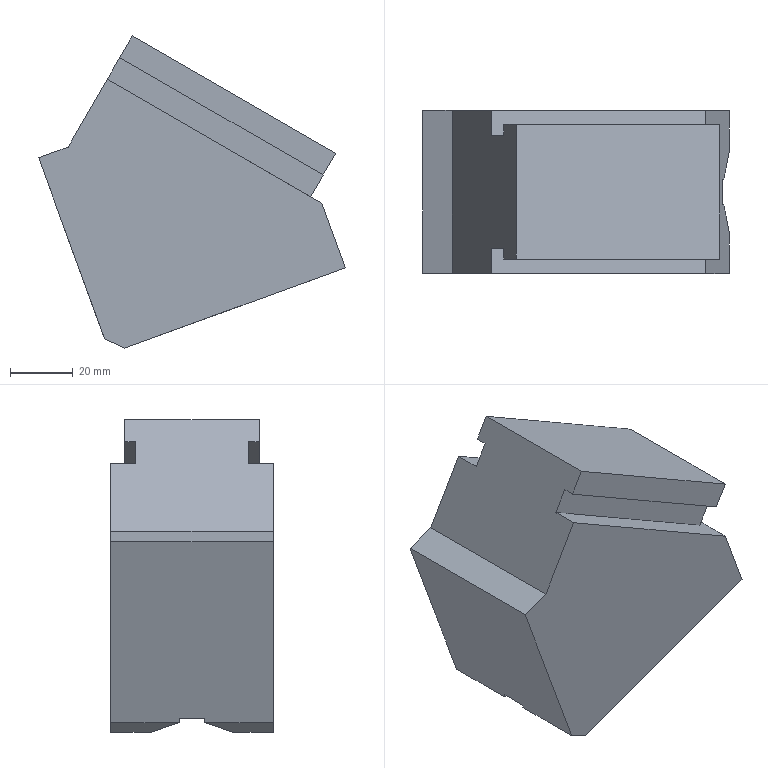Part | NX | features solid 2 | 1 solid | 32 faces | box 97.92 x 52 x 99.707 mm | volume 275545 mm3 | plane 30 | cylinder 2 | commonest cylinder face diameters 20 x2
STEP:
#1=CARTESIAN_POINT('',(-458.531,-112.,17.471));
#2=VERTEX_POINT('',#1);
#3=CARTESIAN_POINT('',(-458.531,-148.,17.471));
#4=VERTEX_POINT('',#3);
#5=CARTESIAN_POINT('',(-458.531,-112.,17.471));
#6=DIRECTION('',(0.,-1.,0.));
#7=VECTOR('',#6,1000.);
#8=LINE('',#5,#7);
#9=EDGE_CURVE('',#2,#4,#8,.T.);
#10=ORIENTED_EDGE('',*,*,#9,.T.);
#11=CARTESIAN_POINT('',(-523.483,-148.,54.971));
#12=VERTEX_POINT('',#11);
#13=CARTESIAN_POINT('',(-458.531,-148.,17.471));
#14=DIRECTION('',(-0.866,0.,0.5));
#15=VECTOR('',#14,1000.);
#16=LINE('',#13,#15);
#17=EDGE_CURVE('',#4,#12,#16,.T.);
#18=ORIENTED_EDGE('',*,*,#17,.T.);
#19=CARTESIAN_POINT('',(-523.483,-156.,54.971));
#20=VERTEX_POINT('',#19);
#21=CARTESIAN_POINT('',(-523.483,-156.,54.971));
#22=DIRECTION('',(0.,1.,0.));
#23=VECTOR('',#22,1000.);
#24=LINE('',#21,#23);
#25=EDGE_CURVE('',#20,#12,#24,.T.);
#26=ORIENTED_EDGE('',*,*,#25,.F.);
#27=CARTESIAN_POINT('',(-454.975,-156.,15.417));
#28=VERTEX_POINT('',#27);
#29=CARTESIAN_POINT('',(-454.975,-156.,15.417));
#30=DIRECTION('',(-0.866,0.,0.5));
#31=VECTOR('',#30,1000.);
#32=LINE('',#29,#31);
#33=EDGE_CURVE('',#28,#20,#32,.T.);
#34=ORIENTED_EDGE('',*,*,#33,.F.);
#35=CARTESIAN_POINT('',(-454.975,-104.,15.417));
#36=VERTEX_POINT('',#35);
#37=CARTESIAN_POINT('',(-454.975,-156.,15.417));
#38=DIRECTION('',(0.,1.,0.));
#39=VECTOR('',#38,1000.);
#40=LINE('',#37,#39);
#41=EDGE_CURVE('',#28,#36,#40,.T.);
#42=ORIENTED_EDGE('',*,*,#41,.T.);
#43=CARTESIAN_POINT('',(-523.483,-104.,54.971));
#44=VERTEX_POINT('',#43);
#45=CARTESIAN_POINT('',(-454.975,-104.,15.417));
#46=DIRECTION('',(-0.866,0.,0.5));
#47=VECTOR('',#46,1000.);
#48=LINE('',#45,#47);
#49=EDGE_CURVE('',#36,#44,#48,.T.);
#50=ORIENTED_EDGE('',*,*,#49,.T.);
#51=CARTESIAN_POINT('',(-523.483,-112.,54.971));
#52=VERTEX_POINT('',#51);
#53=CARTESIAN_POINT('',(-523.483,-156.,54.971));
#54=DIRECTION('',(0.,1.,0.));
#55=VECTOR('',#54,1000.);
#56=LINE('',#53,#55);
#57=EDGE_CURVE('',#52,#44,#56,.T.);
#58=ORIENTED_EDGE('',*,*,#57,.F.);
#59=CARTESIAN_POINT('',(-458.531,-112.,17.471));
#60=DIRECTION('',(-0.866,0.,0.5));
#61=VECTOR('',#60,1000.);
#62=LINE('',#59,#61);
#63=EDGE_CURVE('',#2,#52,#62,.T.);
#64=ORIENTED_EDGE('',*,*,#63,.F.);
#65=EDGE_LOOP('',(#10,#18,#26,#34,#42,#50,#58,#64));
#66=FACE_BOUND('',#65,.T.);
#67=CARTESIAN_POINT('',(-454.975,-156.,15.417));
#68=DIRECTION('',(0.5,0.,0.866));
#69=DIRECTION('',(-0.866,0.,0.5));
#70=AXIS2_PLACEMENT_3D('',#67,#68,#69);
#71=PLANE('',#70);
#72=ADVANCED_FACE('',(#66),#71,.T.);
#73=CARTESIAN_POINT('',(-517.937,-142.99,-30.879));
#74=VERTEX_POINT('',#73);
#75=CARTESIAN_POINT('',(-447.46,-142.99,-5.228));
#76=VERTEX_POINT('',#75);
#77=CARTESIAN_POINT('',(-447.46,-142.99,-5.228));
#78=DIRECTION('',(0.9397,0.,0.342));
#79=VECTOR('',#78,1000.);
#80=LINE('',#77,#79);
#81=EDGE_CURVE('',#74,#76,#80,.T.);
#82=ORIENTED_EDGE('',*,*,#81,.T.);
#83=CARTESIAN_POINT('',(-447.46,-156.,-5.228));
#84=VERTEX_POINT('',#83);
#85=CARTESIAN_POINT('',(-447.46,-156.,-5.228));
#86=DIRECTION('',(0.,1.,0.));
#87=VECTOR('',#86,1000.);
#88=LINE('',#85,#87);
#89=EDGE_CURVE('',#84,#76,#88,.T.);
#90=ORIENTED_EDGE('',*,*,#89,.F.);
#91=CARTESIAN_POINT('',(-517.937,-156.,-30.879));
#92=VERTEX_POINT('',#91);
#93=CARTESIAN_POINT('',(-447.46,-156.,-5.228));
#94=DIRECTION('',(-0.9397,0.,-0.342));
#95=VECTOR('',#94,1000.);
#96=LINE('',#93,#95);
#97=EDGE_CURVE('',#84,#92,#96,.T.);
#98=ORIENTED_EDGE('',*,*,#97,.T.);
#99=CARTESIAN_POINT('',(-517.937,-156.,-30.879));
#100=DIRECTION('',(0.,-1.,0.));
#101=VECTOR('',#100,1000.);
#102=LINE('',#99,#101);
#103=EDGE_CURVE('',#74,#92,#102,.T.);
#104=ORIENTED_EDGE('',*,*,#103,.F.);
#105=EDGE_LOOP('',(#82,#90,#98,#104));
#106=FACE_BOUND('',#105,.T.);
#107=CARTESIAN_POINT('',(-447.46,-156.,-5.228));
#108=DIRECTION('',(-0.342,0.,0.9397));
#109=DIRECTION('',(-0.9397,0.,-0.342));
#110=AXIS2_PLACEMENT_3D('',#107,#108,#109);
#111=PLANE('',#110);
#112=ADVANCED_FACE('',(#106),#111,.F.);
#113=CARTESIAN_POINT('',(-449.236,-134.,-0.3504));
#114=VERTEX_POINT('',#113);
#115=CARTESIAN_POINT('',(-449.236,-134.,-0.3504));
#116=DIRECTION('',(0.171,-0.866,-0.4698));
#117=VECTOR('',#116,1000.);
#118=LINE('',#115,#117);
#119=EDGE_CURVE('',#114,#76,#118,.T.);
#120=ORIENTED_EDGE('',*,*,#119,.F.);
#121=CARTESIAN_POINT('',(-449.683,-134.,0.8801));
#122=VERTEX_POINT('',#121);
#123=CARTESIAN_POINT('',(-449.683,-134.,0.8801));
#124=DIRECTION('',(0.342,0.,-0.9397));
#125=VECTOR('',#124,1000.);
#126=LINE('',#123,#125);
#127=EDGE_CURVE('',#122,#114,#126,.T.);
#128=ORIENTED_EDGE('',*,*,#127,.F.);
#129=CARTESIAN_POINT('',(-449.683,-126.,0.8801));
#130=VERTEX_POINT('',#129);
#131=CARTESIAN_POINT('',(-449.683,-134.,0.8801));
#132=DIRECTION('',(0.,1.,0.));
#133=VECTOR('',#132,1000.);
#134=LINE('',#131,#133);
#135=EDGE_CURVE('',#122,#130,#134,.T.);
#136=ORIENTED_EDGE('',*,*,#135,.T.);
#137=CARTESIAN_POINT('',(-449.236,-126.,-0.3504));
#138=VERTEX_POINT('',#137);
#139=CARTESIAN_POINT('',(-449.236,-126.,-0.3504));
#140=DIRECTION('',(-0.342,0.,0.9397));
#141=VECTOR('',#140,1000.);
#142=LINE('',#139,#141);
#143=EDGE_CURVE('',#138,#130,#142,.T.);
#144=ORIENTED_EDGE('',*,*,#143,.F.);
#145=CARTESIAN_POINT('',(-447.46,-117.01,-5.228));
#146=VERTEX_POINT('',#145);
#147=CARTESIAN_POINT('',(-447.46,-117.01,-5.228));
#148=DIRECTION('',(0.171,0.866,-0.4698));
#149=VECTOR('',#148,1000.);
#150=LINE('',#147,#149);
#151=EDGE_CURVE('',#138,#146,#150,.T.);
#152=ORIENTED_EDGE('',*,*,#151,.T.);
#153=CARTESIAN_POINT('',(-447.46,-104.,-5.228));
#154=VERTEX_POINT('',#153);
#155=CARTESIAN_POINT('',(-447.46,-156.,-5.228));
#156=DIRECTION('',(0.,1.,0.));
#157=VECTOR('',#156,1000.);
#158=LINE('',#155,#157);
#159=EDGE_CURVE('',#146,#154,#158,.T.);
#160=ORIENTED_EDGE('',*,*,#159,.T.);
#161=CARTESIAN_POINT('',(-454.975,-104.,15.417));
#162=DIRECTION('',(0.342,0.,-0.9397));
#163=VECTOR('',#162,1000.);
#164=LINE('',#161,#163);
#165=EDGE_CURVE('',#36,#154,#164,.T.);
#166=ORIENTED_EDGE('',*,*,#165,.F.);
#167=ORIENTED_EDGE('',*,*,#41,.F.);
#168=CARTESIAN_POINT('',(-454.975,-156.,15.417));
#169=DIRECTION('',(0.342,0.,-0.9397));
#170=VECTOR('',#169,1000.);
#171=LINE('',#168,#170);
#172=EDGE_CURVE('',#28,#84,#171,.T.);
#173=ORIENTED_EDGE('',*,*,#172,.T.);
#174=ORIENTED_EDGE('',*,*,#89,.T.);
#175=EDGE_LOOP('',(#120,#128,#136,#144,#152,#160,#166,#167,#173,#174));
#176=FACE_BOUND('',#175,.T.);
#177=CARTESIAN_POINT('',(-454.975,-156.,15.417));
#178=DIRECTION('',(-0.9397,0.,-0.342));
#179=DIRECTION('',(0.342,0.,-0.9397));
#180=AXIS2_PLACEMENT_3D('',#177,#178,#179);
#181=PLANE('',#180);
#182=ADVANCED_FACE('',(#176),#181,.F.);
#183=CARTESIAN_POINT('',(-524.346,-125.67,-27.891));
#184=VERTEX_POINT('',#183);
#185=CARTESIAN_POINT('',(-524.411,-126.,-27.712));
#186=VERTEX_POINT('',#185);
#187=CARTESIAN_POINT('',(-534.096,-175.048,-1.102));
#188=DIRECTION('',(-0.171,-0.866,0.4698));
#189=VECTOR('',#188,1000.);
#190=LINE('',#187,#189);
#191=EDGE_CURVE('',#184,#186,#190,.T.);
#192=ORIENTED_EDGE('',*,*,#191,.T.);
#193=CARTESIAN_POINT('',(-524.859,-126.,-26.482));
#194=VERTEX_POINT('',#193);
#195=CARTESIAN_POINT('',(-545.38,-126.,29.9));
#196=DIRECTION('',(0.342,0.,-0.9397));
#197=VECTOR('',#196,1000.);
#198=LINE('',#195,#197);
#199=EDGE_CURVE('',#194,#186,#198,.T.);
#200=ORIENTED_EDGE('',*,*,#199,.F.);
#201=CARTESIAN_POINT('',(-524.859,-134.,-26.482));
#202=VERTEX_POINT('',#201);
#203=CARTESIAN_POINT('',(-524.859,-156.,-26.482));
#204=DIRECTION('',(0.,-1.,0.));
#205=VECTOR('',#204,1000.);
#206=LINE('',#203,#205);
#207=EDGE_CURVE('',#194,#202,#206,.T.);
#208=ORIENTED_EDGE('',*,*,#207,.T.);
#209=CARTESIAN_POINT('',(-524.411,-134.,-27.712));
#210=VERTEX_POINT('',#209);
#211=CARTESIAN_POINT('',(-545.38,-134.,29.9));
#212=DIRECTION('',(-0.342,0.,0.9397));
#213=VECTOR('',#212,1000.);
#214=LINE('',#211,#213);
#215=EDGE_CURVE('',#210,#202,#214,.T.);
#216=ORIENTED_EDGE('',*,*,#215,.F.);
#217=CARTESIAN_POINT('',(-524.346,-134.33,-27.891));
#218=VERTEX_POINT('',#217);
#219=CARTESIAN_POINT('',(-526.395,-123.952,-22.261));
#220=DIRECTION('',(-0.171,0.866,0.4698));
#221=VECTOR('',#220,1000.);
#222=LINE('',#219,#221);
#223=EDGE_CURVE('',#218,#210,#222,.T.);
#224=ORIENTED_EDGE('',*,*,#223,.F.);
#225=CARTESIAN_POINT('',(-524.346,-156.,-27.891));
#226=VERTEX_POINT('',#225);
#227=CARTESIAN_POINT('',(-524.346,-142.99,-27.891));
#228=DIRECTION('',(0.,1.,0.));
#229=VECTOR('',#228,1000.);
#230=LINE('',#227,#229);
#231=EDGE_CURVE('',#226,#218,#230,.T.);
#232=ORIENTED_EDGE('',*,*,#231,.F.);
#233=CARTESIAN_POINT('',(-545.38,-156.,29.9));
#234=VERTEX_POINT('',#233);
#235=CARTESIAN_POINT('',(-545.38,-156.,29.9));
#236=DIRECTION('',(0.342,0.,-0.9397));
#237=VECTOR('',#236,1000.);
#238=LINE('',#235,#237);
#239=EDGE_CURVE('',#234,#226,#238,.T.);
#240=ORIENTED_EDGE('',*,*,#239,.F.);
#241=CARTESIAN_POINT('',(-545.38,-104.,29.9));
#242=VERTEX_POINT('',#241);
#243=CARTESIAN_POINT('',(-545.38,-156.,29.9));
#244=DIRECTION('',(0.,1.,0.));
#245=VECTOR('',#244,1000.);
#246=LINE('',#243,#245);
#247=EDGE_CURVE('',#234,#242,#246,.T.);
#248=ORIENTED_EDGE('',*,*,#247,.T.);
#249=CARTESIAN_POINT('',(-524.346,-104.,-27.891));
#250=VERTEX_POINT('',#249);
#251=CARTESIAN_POINT('',(-545.38,-104.,29.9));
#252=DIRECTION('',(0.342,0.,-0.9397));
#253=VECTOR('',#252,1000.);
#254=LINE('',#251,#253);
#255=EDGE_CURVE('',#242,#250,#254,.T.);
#256=ORIENTED_EDGE('',*,*,#255,.T.);
#257=CARTESIAN_POINT('',(-524.346,-104.,-27.891));
#258=DIRECTION('',(0.,1.,0.));
#259=VECTOR('',#258,1000.);
#260=LINE('',#257,#259);
#261=EDGE_CURVE('',#184,#250,#260,.T.);
#262=ORIENTED_EDGE('',*,*,#261,.F.);
#263=EDGE_LOOP('',(#192,#200,#208,#216,#224,#232,#240,#248,#256,#262));
#264=FACE_BOUND('',#263,.T.);
#265=CARTESIAN_POINT('',(-545.38,-156.,29.9));
#266=DIRECTION('',(-0.9397,0.,-0.342));
#267=DIRECTION('',(0.342,0.,-0.9397));
#268=AXIS2_PLACEMENT_3D('',#265,#266,#267);
#269=PLANE('',#268);
#270=ADVANCED_FACE('',(#264),#269,.T.);
#271=ORIENTED_EDGE('',*,*,#255,.F.);
#272=CARTESIAN_POINT('',(-535.983,-104.,33.32));
#273=VERTEX_POINT('',#272);
#274=CARTESIAN_POINT('',(-535.983,-104.,33.32));
#275=DIRECTION('',(-0.9397,0.,-0.342));
#276=VECTOR('',#275,1000.);
#277=LINE('',#274,#276);
#278=EDGE_CURVE('',#273,#242,#277,.T.);
#279=ORIENTED_EDGE('',*,*,#278,.F.);
#280=CARTESIAN_POINT('',(-523.483,-104.,54.971));
#281=DIRECTION('',(-0.5,0.,-0.866));
#282=VECTOR('',#281,1000.);
#283=LINE('',#280,#282);
#284=EDGE_CURVE('',#44,#273,#283,.T.);
#285=ORIENTED_EDGE('',*,*,#284,.F.);
#286=ORIENTED_EDGE('',*,*,#49,.F.);
#287=ORIENTED_EDGE('',*,*,#165,.T.);
#288=CARTESIAN_POINT('',(-473.862,-104.,-14.837));
#289=VERTEX_POINT('',#288);
#290=CARTESIAN_POINT('',(-447.46,-104.,-5.228));
#291=DIRECTION('',(-0.9397,0.,-0.342));
#292=VECTOR('',#291,1000.);
#293=LINE('',#290,#292);
#294=EDGE_CURVE('',#154,#289,#293,.T.);
#295=ORIENTED_EDGE('',*,*,#294,.T.);
#296=CARTESIAN_POINT('',(-479.59,-104.,0.8997));
#297=VERTEX_POINT('',#296);
#298=CARTESIAN_POINT('',(-486.43,-104.,19.694));
#299=DIRECTION('',(0.342,0.,-0.9397));
#300=VECTOR('',#299,1000.);
#301=LINE('',#298,#300);
#302=EDGE_CURVE('',#297,#289,#301,.T.);
#303=ORIENTED_EDGE('',*,*,#302,.F.);
#304=CARTESIAN_POINT('',(-486.43,-104.,19.694));
#305=VERTEX_POINT('',#304);
#306=CARTESIAN_POINT('',(-483.01,-104.,10.297));
#307=DIRECTION('',(0.,1.,0.));
#308=DIRECTION('',(-1.,0.,0.));
#309=AXIS2_PLACEMENT_3D('',#306,#307,#308);
#310=CIRCLE('',#309,10.);
#311=EDGE_CURVE('',#305,#297,#310,.T.);
#312=ORIENTED_EDGE('',*,*,#311,.F.);
#313=CARTESIAN_POINT('',(-505.224,-104.,12.853));
#314=VERTEX_POINT('',#313);
#315=CARTESIAN_POINT('',(-505.224,-104.,12.853));
#316=DIRECTION('',(0.9397,0.,0.342));
#317=VECTOR('',#316,1000.);
#318=LINE('',#315,#317);
#319=EDGE_CURVE('',#314,#305,#318,.T.);
#320=ORIENTED_EDGE('',*,*,#319,.F.);
#321=CARTESIAN_POINT('',(-498.383,-104.,-5.941));
#322=VERTEX_POINT('',#321);
#323=CARTESIAN_POINT('',(-501.804,-104.,3.456));
#324=DIRECTION('',(0.,1.,0.));
#325=DIRECTION('',(-1.,0.,0.));
#326=AXIS2_PLACEMENT_3D('',#323,#324,#325);
#327=CIRCLE('',#326,10.);
#328=EDGE_CURVE('',#322,#314,#327,.T.);
#329=ORIENTED_EDGE('',*,*,#328,.F.);
#330=CARTESIAN_POINT('',(-492.656,-104.,-21.678));
#331=VERTEX_POINT('',#330);
#332=CARTESIAN_POINT('',(-505.224,-104.,12.853));
#333=DIRECTION('',(0.342,0.,-0.9397));
#334=VECTOR('',#333,1000.);
#335=LINE('',#332,#334);
#336=EDGE_CURVE('',#322,#331,#335,.T.);
#337=ORIENTED_EDGE('',*,*,#336,.T.);
#338=CARTESIAN_POINT('',(-517.937,-104.,-30.879));
#339=VERTEX_POINT('',#338);
#340=CARTESIAN_POINT('',(-447.46,-104.,-5.228));
#341=DIRECTION('',(-0.9397,0.,-0.342));
#342=VECTOR('',#341,1000.);
#343=LINE('',#340,#342);
#344=EDGE_CURVE('',#331,#339,#343,.T.);
#345=ORIENTED_EDGE('',*,*,#344,.T.);
#346=CARTESIAN_POINT('',(-524.346,-104.,-27.891));
#347=DIRECTION('',(0.9063,0.,-0.4226));
#348=VECTOR('',#347,1000.);
#349=LINE('',#346,#348);
#350=EDGE_CURVE('',#250,#339,#349,.T.);
#351=ORIENTED_EDGE('',*,*,#350,.F.);
#352=EDGE_LOOP('',(#271,#279,#285,#286,#287,#295,#303,#312,#320,#329,#337,#345,#351));
#353=FACE_BOUND('',#352,.T.);
#354=CARTESIAN_POINT('',(-447.46,-104.,-5.228));
#355=DIRECTION('',(0.,-1.,0.));
#356=DIRECTION('',(0.,0.,-1.));
#357=AXIS2_PLACEMENT_3D('',#354,#355,#356);
#358=PLANE('',#357);
#359=ADVANCED_FACE('',(#353),#358,.F.);
#360=ORIENTED_EDGE('',*,*,#344,.F.);
#361=CARTESIAN_POINT('',(-492.656,-110.,-21.678));
#362=VERTEX_POINT('',#361);
#363=CARTESIAN_POINT('',(-492.656,-156.,-21.678));
#364=DIRECTION('',(0.,1.,0.));
#365=VECTOR('',#364,1000.);
#366=LINE('',#363,#365);
#367=EDGE_CURVE('',#362,#331,#366,.T.);
#368=ORIENTED_EDGE('',*,*,#367,.F.);
#369=CARTESIAN_POINT('',(-473.862,-110.,-14.837));
#370=VERTEX_POINT('',#369);
#371=CARTESIAN_POINT('',(-447.46,-110.,-5.228));
#372=DIRECTION('',(0.9397,0.,0.342));
#373=VECTOR('',#372,1000.);
#374=LINE('',#371,#373);
#375=EDGE_CURVE('',#362,#370,#374,.T.);
#376=ORIENTED_EDGE('',*,*,#375,.T.);
#377=CARTESIAN_POINT('',(-473.862,-156.,-14.837));
#378=DIRECTION('',(0.,1.,0.));
#379=VECTOR('',#378,1000.);
#380=LINE('',#377,#379);
#381=EDGE_CURVE('',#370,#289,#380,.T.);
#382=ORIENTED_EDGE('',*,*,#381,.T.);
#383=ORIENTED_EDGE('',*,*,#294,.F.);
#384=ORIENTED_EDGE('',*,*,#159,.F.);
#385=CARTESIAN_POINT('',(-517.937,-117.01,-30.879));
#386=VERTEX_POINT('',#385);
#387=CARTESIAN_POINT('',(-447.46,-117.01,-5.228));
#388=DIRECTION('',(0.9397,0.,0.342));
#389=VECTOR('',#388,1000.);
#390=LINE('',#387,#389);
#391=EDGE_CURVE('',#386,#146,#390,.T.);
#392=ORIENTED_EDGE('',*,*,#391,.F.);
#393=CARTESIAN_POINT('',(-517.937,-117.01,-30.879));
#394=DIRECTION('',(0.,-1.,0.));
#395=VECTOR('',#394,1000.);
#396=LINE('',#393,#395);
#397=EDGE_CURVE('',#339,#386,#396,.T.);
#398=ORIENTED_EDGE('',*,*,#397,.F.);
#399=EDGE_LOOP('',(#360,#368,#376,#382,#383,#384,#392,#398));
#400=FACE_BOUND('',#399,.T.);
#401=CARTESIAN_POINT('',(-447.46,-156.,-5.228));
#402=DIRECTION('',(-0.342,0.,0.9397));
#403=DIRECTION('',(-0.9397,0.,-0.342));
#404=AXIS2_PLACEMENT_3D('',#401,#402,#403);
#405=PLANE('',#404);
#406=ADVANCED_FACE('',(#400),#405,.F.);
#407=CARTESIAN_POINT('',(-498.383,-110.,-5.941));
#408=VERTEX_POINT('',#407);
#409=CARTESIAN_POINT('',(-479.59,-110.,0.8997));
#410=VERTEX_POINT('',#409);
#411=CARTESIAN_POINT('',(-498.383,-110.,-5.941));
#412=DIRECTION('',(0.9397,0.,0.342));
#413=VECTOR('',#412,1000.);
#414=LINE('',#411,#413);
#415=EDGE_CURVE('',#408,#410,#414,.T.);
#416=ORIENTED_EDGE('',*,*,#415,.F.);
#417=CARTESIAN_POINT('',(-498.383,-116.,-5.941));
#418=VERTEX_POINT('',#417);
#419=CARTESIAN_POINT('',(-498.383,-116.,-5.941));
#420=DIRECTION('',(0.,1.,0.));
#421=VECTOR('',#420,1000.);
#422=LINE('',#419,#421);
#423=EDGE_CURVE('',#418,#408,#422,.T.);
#424=ORIENTED_EDGE('',*,*,#423,.F.);
#425=CARTESIAN_POINT('',(-479.59,-116.,0.8997));
#426=VERTEX_POINT('',#425);
#427=CARTESIAN_POINT('',(-498.383,-116.,-5.941));
#428=DIRECTION('',(0.9397,0.,0.342));
#429=VECTOR('',#428,1000.);
#430=LINE('',#427,#429);
#431=EDGE_CURVE('',#418,#426,#430,.T.);
#432=ORIENTED_EDGE('',*,*,#431,.T.);
#433=CARTESIAN_POINT('',(-479.59,-116.,0.8997));
#434=DIRECTION('',(0.,1.,0.));
#435=VECTOR('',#434,1000.);
#436=LINE('',#433,#435);
#437=EDGE_CURVE('',#426,#410,#436,.T.);
#438=ORIENTED_EDGE('',*,*,#437,.T.);
#439=EDGE_LOOP('',(#416,#424,#432,#438));
#440=FACE_BOUND('',#439,.T.);
#441=CARTESIAN_POINT('',(-498.383,-116.,-5.941));
#442=DIRECTION('',(0.342,0.,-0.9397));
#443=DIRECTION('',(0.9397,0.,0.342));
#444=AXIS2_PLACEMENT_3D('',#441,#442,#443);
#445=PLANE('',#444);
#446=ADVANCED_FACE('',(#440),#445,.F.);
#447=ORIENTED_EDGE('',*,*,#278,.T.);
#448=ORIENTED_EDGE('',*,*,#247,.F.);
#449=CARTESIAN_POINT('',(-535.983,-156.,33.32));
#450=VERTEX_POINT('',#449);
#451=CARTESIAN_POINT('',(-535.983,-156.,33.32));
#452=DIRECTION('',(-0.9397,0.,-0.342));
#453=VECTOR('',#452,1000.);
#454=LINE('',#451,#453);
#455=EDGE_CURVE('',#450,#234,#454,.T.);
#456=ORIENTED_EDGE('',*,*,#455,.F.);
#457=CARTESIAN_POINT('',(-535.983,-156.,33.32));
#458=DIRECTION('',(0.,1.,0.));
#459=VECTOR('',#458,1000.);
#460=LINE('',#457,#459);
#461=EDGE_CURVE('',#450,#273,#460,.T.);
#462=ORIENTED_EDGE('',*,*,#461,.T.);
#463=EDGE_LOOP('',(#447,#448,#456,#462));
#464=FACE_BOUND('',#463,.T.);
#465=CARTESIAN_POINT('',(-535.983,-156.,33.32));
#466=DIRECTION('',(-0.342,0.,0.9397));
#467=DIRECTION('',(-0.9397,0.,-0.342));
#468=AXIS2_PLACEMENT_3D('',#465,#466,#467);
#469=PLANE('',#468);
#470=ADVANCED_FACE('',(#464),#469,.T.);
#471=ORIENTED_EDGE('',*,*,#284,.T.);
#472=ORIENTED_EDGE('',*,*,#461,.F.);
#473=CARTESIAN_POINT('',(-523.483,-156.,54.971));
#474=DIRECTION('',(-0.5,0.,-0.866));
#475=VECTOR('',#474,1000.);
#476=LINE('',#473,#475);
#477=EDGE_CURVE('',#20,#450,#476,.T.);
#478=ORIENTED_EDGE('',*,*,#477,.F.);
#479=ORIENTED_EDGE('',*,*,#25,.T.);
#480=CARTESIAN_POINT('',(-519.483,-148.,61.899));
#481=VERTEX_POINT('',#480);
#482=CARTESIAN_POINT('',(-519.483,-148.,61.899));
#483=DIRECTION('',(-0.5,0.,-0.866));
#484=VECTOR('',#483,1000.);
#485=LINE('',#482,#484);
#486=EDGE_CURVE('',#481,#12,#485,.T.);
#487=ORIENTED_EDGE('',*,*,#486,.F.);
#488=CARTESIAN_POINT('',(-519.483,-151.5,61.899));
#489=VERTEX_POINT('',#488);
#490=CARTESIAN_POINT('',(-519.483,-108.5,61.899));
#491=DIRECTION('',(0.,-1.,0.));
#492=VECTOR('',#491,1000.);
#493=LINE('',#490,#492);
#494=EDGE_CURVE('',#481,#489,#493,.T.);
#495=ORIENTED_EDGE('',*,*,#494,.T.);
#496=CARTESIAN_POINT('',(-515.483,-151.5,68.827));
#497=VERTEX_POINT('',#496);
#498=CARTESIAN_POINT('',(-515.483,-151.5,68.827));
#499=DIRECTION('',(-0.5,0.,-0.866));
#500=VECTOR('',#499,1000.);
#501=LINE('',#498,#500);
#502=EDGE_CURVE('',#497,#489,#501,.T.);
#503=ORIENTED_EDGE('',*,*,#502,.F.);
#504=CARTESIAN_POINT('',(-515.483,-108.5,68.827));
#505=VERTEX_POINT('',#504);
#506=CARTESIAN_POINT('',(-515.483,-108.5,68.827));
#507=DIRECTION('',(0.,-1.,0.));
#508=VECTOR('',#507,1000.);
#509=LINE('',#506,#508);
#510=EDGE_CURVE('',#505,#497,#509,.T.);
#511=ORIENTED_EDGE('',*,*,#510,.F.);
#512=CARTESIAN_POINT('',(-519.483,-108.5,61.899));
#513=VERTEX_POINT('',#512);
#514=CARTESIAN_POINT('',(-515.483,-108.5,68.827));
#515=DIRECTION('',(-0.5,0.,-0.866));
#516=VECTOR('',#515,1000.);
#517=LINE('',#514,#516);
#518=EDGE_CURVE('',#505,#513,#517,.T.);
#519=ORIENTED_EDGE('',*,*,#518,.T.);
#520=CARTESIAN_POINT('',(-519.483,-112.,61.899));
#521=VERTEX_POINT('',#520);
#522=CARTESIAN_POINT('',(-519.483,-108.5,61.899));
#523=DIRECTION('',(0.,-1.,0.));
#524=VECTOR('',#523,1000.);
#525=LINE('',#522,#524);
#526=EDGE_CURVE('',#513,#521,#525,.T.);
#527=ORIENTED_EDGE('',*,*,#526,.T.);
#528=CARTESIAN_POINT('',(-519.483,-112.,61.899));
#529=DIRECTION('',(-0.5,0.,-0.866));
#530=VECTOR('',#529,1000.);
#531=LINE('',#528,#530);
#532=EDGE_CURVE('',#521,#52,#531,.T.);
#533=ORIENTED_EDGE('',*,*,#532,.T.);
#534=ORIENTED_EDGE('',*,*,#57,.T.);
#535=EDGE_LOOP('',(#471,#472,#478,#479,#487,#495,#503,#511,#519,#527,#533,#534));
#536=FACE_BOUND('',#535,.T.);
#537=CARTESIAN_POINT('',(-523.483,-156.,54.971));
#538=DIRECTION('',(-0.866,0.,0.5));
#539=DIRECTION('',(-0.5,0.,-0.866));
#540=AXIS2_PLACEMENT_3D('',#537,#538,#539);
#541=PLANE('',#540);
#542=ADVANCED_FACE('',(#536),#541,.T.);
#543=ORIENTED_EDGE('',*,*,#97,.F.);
#544=ORIENTED_EDGE('',*,*,#172,.F.);
#545=ORIENTED_EDGE('',*,*,#33,.T.);
#546=ORIENTED_EDGE('',*,*,#477,.T.);
#547=ORIENTED_EDGE('',*,*,#455,.T.);
#548=ORIENTED_EDGE('',*,*,#239,.T.);
#549=CARTESIAN_POINT('',(-469.873,-156.,-53.292));
#550=DIRECTION('',(-0.9063,0.,0.4226));
#551=VECTOR('',#550,1000.);
#552=LINE('',#549,#551);
#553=EDGE_CURVE('',#92,#226,#552,.T.);
#554=ORIENTED_EDGE('',*,*,#553,.F.);
#555=EDGE_LOOP('',(#543,#544,#545,#546,#547,#548,#554));
#556=FACE_BOUND('',#555,.T.);
#557=CARTESIAN_POINT('',(-447.46,-156.,-5.228));
#558=DIRECTION('',(0.,-1.,0.));
#559=DIRECTION('',(0.,0.,-1.));
#560=AXIS2_PLACEMENT_3D('',#557,#558,#559);
#561=PLANE('',#560);
#562=ADVANCED_FACE('',(#556),#561,.T.);
#563=ORIENTED_EDGE('',*,*,#319,.T.);
#564=CARTESIAN_POINT('',(-486.43,-116.,19.694));
#565=VERTEX_POINT('',#564);
#566=CARTESIAN_POINT('',(-486.43,-116.,19.694));
#567=DIRECTION('',(0.,1.,0.));
#568=VECTOR('',#567,1000.);
#569=LINE('',#566,#568);
#570=EDGE_CURVE('',#565,#305,#569,.T.);
#571=ORIENTED_EDGE('',*,*,#570,.F.);
#572=CARTESIAN_POINT('',(-505.224,-116.,12.853));
#573=VERTEX_POINT('',#572);
#574=CARTESIAN_POINT('',(-505.224,-116.,12.853));
#575=DIRECTION('',(0.9397,0.,0.342));
#576=VECTOR('',#575,1000.);
#577=LINE('',#574,#576);
#578=EDGE_CURVE('',#573,#565,#577,.T.);
#579=ORIENTED_EDGE('',*,*,#578,.F.);
#580=CARTESIAN_POINT('',(-505.224,-116.,12.853));
#581=DIRECTION('',(0.,1.,0.));
#582=VECTOR('',#581,1000.);
#583=LINE('',#580,#582);
#584=EDGE_CURVE('',#573,#314,#583,.T.);
#585=ORIENTED_EDGE('',*,*,#584,.T.);
#586=EDGE_LOOP('',(#563,#571,#579,#585));
#587=FACE_BOUND('',#586,.T.);
#588=CARTESIAN_POINT('',(-505.224,-116.,12.853));
#589=DIRECTION('',(0.342,0.,-0.9397));
#590=DIRECTION('',(0.9397,0.,0.342));
#591=AXIS2_PLACEMENT_3D('',#588,#589,#590);
#592=PLANE('',#591);
#593=ADVANCED_FACE('',(#587),#592,.T.);
#594=ORIENTED_EDGE('',*,*,#311,.T.);
#595=CARTESIAN_POINT('',(-479.59,-116.,0.8997));
#596=DIRECTION('',(0.,-1.,0.));
#597=VECTOR('',#596,1000.);
#598=LINE('',#595,#597);
#599=EDGE_CURVE('',#297,#410,#598,.T.);
#600=ORIENTED_EDGE('',*,*,#599,.T.);
#601=ORIENTED_EDGE('',*,*,#437,.F.);
#602=CARTESIAN_POINT('',(-483.01,-116.,10.297));
#603=DIRECTION('',(0.,1.,0.));
#604=DIRECTION('',(-1.,0.,0.));
#605=AXIS2_PLACEMENT_3D('',#602,#603,#604);
#606=CIRCLE('',#605,10.);
#607=EDGE_CURVE('',#565,#426,#606,.T.);
#608=ORIENTED_EDGE('',*,*,#607,.F.);
#609=ORIENTED_EDGE('',*,*,#570,.T.);
#610=EDGE_LOOP('',(#594,#600,#601,#608,#609));
#611=FACE_BOUND('',#610,.T.);
#612=CARTESIAN_POINT('',(-483.01,-116.,10.297));
#613=DIRECTION('',(0.,1.,0.));
#614=DIRECTION('',(0.,0.,1.));
#615=AXIS2_PLACEMENT_3D('',#612,#613,#614);
#616=CYLINDRICAL_SURFACE('',#615,10.);
#617=ADVANCED_FACE('',(#611),#616,.F.);
#618=ORIENTED_EDGE('',*,*,#328,.T.);
#619=ORIENTED_EDGE('',*,*,#584,.F.);
#620=CARTESIAN_POINT('',(-501.804,-116.,3.456));
#621=DIRECTION('',(0.,1.,0.));
#622=DIRECTION('',(-1.,0.,0.));
#623=AXIS2_PLACEMENT_3D('',#620,#621,#622);
#624=CIRCLE('',#623,10.);
#625=EDGE_CURVE('',#418,#573,#624,.T.);
#626=ORIENTED_EDGE('',*,*,#625,.F.);
#627=ORIENTED_EDGE('',*,*,#423,.T.);
#628=CARTESIAN_POINT('',(-498.383,-116.,-5.941));
#629=DIRECTION('',(0.,1.,0.));
#630=VECTOR('',#629,1000.);
#631=LINE('',#628,#630);
#632=EDGE_CURVE('',#408,#322,#631,.T.);
#633=ORIENTED_EDGE('',*,*,#632,.T.);
#634=EDGE_LOOP('',(#618,#619,#626,#627,#633));
#635=FACE_BOUND('',#634,.T.);
#636=CARTESIAN_POINT('',(-501.804,-116.,3.456));
#637=DIRECTION('',(0.,1.,0.));
#638=DIRECTION('',(0.,0.,1.));
#639=AXIS2_PLACEMENT_3D('',#636,#637,#638);
#640=CYLINDRICAL_SURFACE('',#639,10.);
#641=ADVANCED_FACE('',(#635),#640,.F.);
#642=ORIENTED_EDGE('',*,*,#625,.T.);
#643=ORIENTED_EDGE('',*,*,#578,.T.);
#644=ORIENTED_EDGE('',*,*,#607,.T.);
#645=ORIENTED_EDGE('',*,*,#431,.F.);
#646=EDGE_LOOP('',(#642,#643,#644,#645));
#647=FACE_BOUND('',#646,.T.);
#648=CARTESIAN_POINT('',(-483.01,-116.,10.297));
#649=DIRECTION('',(0.,-1.,0.));
#650=DIRECTION('',(0.,0.,-1.));
#651=AXIS2_PLACEMENT_3D('',#648,#649,#650);
#652=PLANE('',#651);
#653=ADVANCED_FACE('',(#647),#652,.F.);
#654=ORIENTED_EDGE('',*,*,#375,.F.);
#655=CARTESIAN_POINT('',(-490.517,-110.,-27.554));
#656=DIRECTION('',(-0.342,0.,0.9397));
#657=VECTOR('',#656,1000.);
#658=LINE('',#655,#657);
#659=EDGE_CURVE('',#362,#408,#658,.T.);
#660=ORIENTED_EDGE('',*,*,#659,.T.);
#661=ORIENTED_EDGE('',*,*,#415,.T.);
#662=CARTESIAN_POINT('',(-471.723,-110.,-20.713));
#663=DIRECTION('',(-0.342,0.,0.9397));
#664=VECTOR('',#663,1000.);
#665=LINE('',#662,#664);
#666=EDGE_CURVE('',#370,#410,#665,.T.);
#667=ORIENTED_EDGE('',*,*,#666,.F.);
#668=EDGE_LOOP('',(#654,#660,#661,#667));
#669=FACE_BOUND('',#668,.T.);
#670=CARTESIAN_POINT('',(-471.723,-110.,-20.713));
#671=DIRECTION('',(0.,1.,0.));
#672=DIRECTION('',(0.,0.,1.));
#673=AXIS2_PLACEMENT_3D('',#670,#671,#672);
#674=PLANE('',#673);
#675=ADVANCED_FACE('',(#669),#674,.T.);
#676=ORIENTED_EDGE('',*,*,#381,.F.);
#677=ORIENTED_EDGE('',*,*,#666,.T.);
#678=ORIENTED_EDGE('',*,*,#599,.F.);
#679=ORIENTED_EDGE('',*,*,#302,.T.);
#680=EDGE_LOOP('',(#676,#677,#678,#679));
#681=FACE_BOUND('',#680,.T.);
#682=CARTESIAN_POINT('',(-486.43,-110.,19.694));
#683=DIRECTION('',(-0.9397,0.,-0.342));
#684=DIRECTION('',(-0.342,0.,0.9397));
#685=AXIS2_PLACEMENT_3D('',#682,#683,#684);
#686=PLANE('',#685);
#687=ADVANCED_FACE('',(#681),#686,.T.);
#688=ORIENTED_EDGE('',*,*,#659,.F.);
#689=ORIENTED_EDGE('',*,*,#367,.T.);
#690=ORIENTED_EDGE('',*,*,#336,.F.);
#691=ORIENTED_EDGE('',*,*,#632,.F.);
#692=EDGE_LOOP('',(#688,#689,#690,#691));
#693=FACE_BOUND('',#692,.T.);
#694=CARTESIAN_POINT('',(-505.224,-110.,12.853));
#695=DIRECTION('',(-0.9397,0.,-0.342));
#696=DIRECTION('',(-0.342,0.,0.9397));
#697=AXIS2_PLACEMENT_3D('',#694,#695,#696);
#698=PLANE('',#697);
#699=ADVANCED_FACE('',(#693),#698,.F.);
#700=ORIENTED_EDGE('',*,*,#223,.T.);
#701=CARTESIAN_POINT('',(-533.808,-134.,-31.132));
#702=DIRECTION('',(0.9397,0.,0.342));
#703=VECTOR('',#702,1000.);
#704=LINE('',#701,#703);
#705=EDGE_CURVE('',#210,#114,#704,.T.);
#706=ORIENTED_EDGE('',*,*,#705,.T.);
#707=ORIENTED_EDGE('',*,*,#119,.T.);
#708=ORIENTED_EDGE('',*,*,#81,.F.);
#709=CARTESIAN_POINT('',(-527.105,-130.602,-26.605));
#710=DIRECTION('',(0.5732,-0.7746,-0.2673));
#711=VECTOR('',#710,1000.);
#712=LINE('',#709,#711);
#713=EDGE_CURVE('',#218,#74,#712,.T.);
#714=ORIENTED_EDGE('',*,*,#713,.F.);
#715=EDGE_LOOP('',(#700,#706,#707,#708,#714));
#716=FACE_BOUND('',#715,.T.);
#717=CARTESIAN_POINT('',(-533.808,-134.,-31.132));
#718=DIRECTION('',(0.2962,0.5,-0.8138));
#719=DIRECTION('',(0.,0.852,0.5235));
#720=AXIS2_PLACEMENT_3D('',#717,#718,#719);
#721=PLANE('',#720);
#722=ADVANCED_FACE('',(#716),#721,.T.);
#723=ORIENTED_EDGE('',*,*,#391,.T.);
#724=ORIENTED_EDGE('',*,*,#151,.F.);
#725=CARTESIAN_POINT('',(-533.808,-126.,-31.132));
#726=DIRECTION('',(0.9397,0.,0.342));
#727=VECTOR('',#726,1000.);
#728=LINE('',#725,#727);
#729=EDGE_CURVE('',#186,#138,#728,.T.);
#730=ORIENTED_EDGE('',*,*,#729,.F.);
#731=ORIENTED_EDGE('',*,*,#191,.F.);
#732=CARTESIAN_POINT('',(-537.812,-143.868,-21.612));
#733=DIRECTION('',(-0.5732,-0.7746,0.2673));
#734=VECTOR('',#733,1000.);
#735=LINE('',#732,#734);
#736=EDGE_CURVE('',#386,#184,#735,.T.);
#737=ORIENTED_EDGE('',*,*,#736,.F.);
#738=EDGE_LOOP('',(#723,#724,#730,#731,#737));
#739=FACE_BOUND('',#738,.T.);
#740=CARTESIAN_POINT('',(-532.033,-117.01,-36.01));
#741=DIRECTION('',(-0.2962,0.5,0.8138));
#742=DIRECTION('',(0.,-0.852,0.5235));
#743=AXIS2_PLACEMENT_3D('',#740,#741,#742);
#744=PLANE('',#743);
#745=ADVANCED_FACE('',(#739),#744,.F.);
#746=ORIENTED_EDGE('',*,*,#215,.T.);
#747=CARTESIAN_POINT('',(-534.256,-134.,-29.902));
#748=DIRECTION('',(0.9397,0.,0.342));
#749=VECTOR('',#748,1000.);
#750=LINE('',#747,#749);
#751=EDGE_CURVE('',#202,#122,#750,.T.);
#752=ORIENTED_EDGE('',*,*,#751,.T.);
#753=ORIENTED_EDGE('',*,*,#127,.T.);
#754=ORIENTED_EDGE('',*,*,#705,.F.);
#755=EDGE_LOOP('',(#746,#752,#753,#754));
#756=FACE_BOUND('',#755,.T.);
#757=CARTESIAN_POINT('',(-534.256,-134.,-29.902));
#758=DIRECTION('',(0.,1.,0.));
#759=DIRECTION('',(0.,0.,1.));
#760=AXIS2_PLACEMENT_3D('',#757,#758,#759);
#761=PLANE('',#760);
#762=ADVANCED_FACE('',(#756),#761,.T.);
#763=ORIENTED_EDGE('',*,*,#199,.T.);
#764=ORIENTED_EDGE('',*,*,#729,.T.);
#765=ORIENTED_EDGE('',*,*,#143,.T.);
#766=CARTESIAN_POINT('',(-534.256,-126.,-29.902));
#767=DIRECTION('',(0.9397,0.,0.342));
#768=VECTOR('',#767,1000.);
#769=LINE('',#766,#768);
#770=EDGE_CURVE('',#194,#130,#769,.T.);
#771=ORIENTED_EDGE('',*,*,#770,.F.);
#772=EDGE_LOOP('',(#763,#764,#765,#771));
#773=FACE_BOUND('',#772,.T.);
#774=CARTESIAN_POINT('',(-533.808,-126.,-31.132));
#775=DIRECTION('',(0.,-1.,0.));
#776=DIRECTION('',(0.,0.,-1.));
#777=AXIS2_PLACEMENT_3D('',#774,#775,#776);
#778=PLANE('',#777);
#779=ADVANCED_FACE('',(#773),#778,.T.);
#780=ORIENTED_EDGE('',*,*,#770,.T.);
#781=ORIENTED_EDGE('',*,*,#135,.F.);
#782=ORIENTED_EDGE('',*,*,#751,.F.);
#783=ORIENTED_EDGE('',*,*,#207,.F.);
#784=EDGE_LOOP('',(#780,#781,#782,#783));
#785=FACE_BOUND('',#784,.T.);
#786=CARTESIAN_POINT('',(-534.256,-134.,-29.902));
#787=DIRECTION('',(-0.342,0.,0.9397));
#788=DIRECTION('',(-0.9397,0.,-0.342));
#789=AXIS2_PLACEMENT_3D('',#786,#787,#788);
#790=PLANE('',#789);
#791=ADVANCED_FACE('',(#785),#790,.F.);
#792=CARTESIAN_POINT('',(-454.531,-148.,24.399));
#793=VERTEX_POINT('',#792);
#794=CARTESIAN_POINT('',(-454.531,-148.,24.399));
#795=DIRECTION('',(-0.5,0.,-0.866));
#796=VECTOR('',#795,1000.);
#797=LINE('',#794,#796);
#798=EDGE_CURVE('',#793,#4,#797,.T.);
#799=ORIENTED_EDGE('',*,*,#798,.T.);
#800=ORIENTED_EDGE('',*,*,#9,.F.);
#801=CARTESIAN_POINT('',(-454.531,-112.,24.399));
#802=VERTEX_POINT('',#801);
#803=CARTESIAN_POINT('',(-454.531,-112.,24.399));
#804=DIRECTION('',(-0.5,0.,-0.866));
#805=VECTOR('',#804,1000.);
#806=LINE('',#803,#805);
#807=EDGE_CURVE('',#802,#2,#806,.T.);
#808=ORIENTED_EDGE('',*,*,#807,.F.);
#809=CARTESIAN_POINT('',(-454.531,-108.5,24.399));
#810=VERTEX_POINT('',#809);
#811=CARTESIAN_POINT('',(-454.531,-108.5,24.399));
#812=DIRECTION('',(0.,-1.,0.));
#813=VECTOR('',#812,1000.);
#814=LINE('',#811,#813);
#815=EDGE_CURVE('',#810,#802,#814,.T.);
#816=ORIENTED_EDGE('',*,*,#815,.F.);
#817=CARTESIAN_POINT('',(-450.531,-108.5,31.327));
#818=VERTEX_POINT('',#817);
#819=CARTESIAN_POINT('',(-450.531,-108.5,31.327));
#820=DIRECTION('',(-0.5,0.,-0.866));
#821=VECTOR('',#820,1000.);
#822=LINE('',#819,#821);
#823=EDGE_CURVE('',#818,#810,#822,.T.);
#824=ORIENTED_EDGE('',*,*,#823,.F.);
#825=CARTESIAN_POINT('',(-450.531,-151.5,31.327));
#826=VERTEX_POINT('',#825);
#827=CARTESIAN_POINT('',(-450.531,-108.5,31.327));
#828=DIRECTION('',(0.,-1.,0.));
#829=VECTOR('',#828,1000.);
#830=LINE('',#827,#829);
#831=EDGE_CURVE('',#818,#826,#830,.T.);
#832=ORIENTED_EDGE('',*,*,#831,.T.);
#833=CARTESIAN_POINT('',(-454.531,-151.5,24.399));
#834=VERTEX_POINT('',#833);
#835=CARTESIAN_POINT('',(-450.531,-151.5,31.327));
#836=DIRECTION('',(-0.5,0.,-0.866));
#837=VECTOR('',#836,1000.);
#838=LINE('',#835,#837);
#839=EDGE_CURVE('',#826,#834,#838,.T.);
#840=ORIENTED_EDGE('',*,*,#839,.T.);
#841=CARTESIAN_POINT('',(-454.531,-108.5,24.399));
#842=DIRECTION('',(0.,-1.,0.));
#843=VECTOR('',#842,1000.);
#844=LINE('',#841,#843);
#845=EDGE_CURVE('',#793,#834,#844,.T.);
#846=ORIENTED_EDGE('',*,*,#845,.F.);
#847=EDGE_LOOP('',(#799,#800,#808,#816,#824,#832,#840,#846));
#848=FACE_BOUND('',#847,.T.);
#849=CARTESIAN_POINT('',(-454.531,-112.,24.399));
#850=DIRECTION('',(0.866,0.,-0.5));
#851=DIRECTION('',(0.5,0.,0.866));
#852=AXIS2_PLACEMENT_3D('',#849,#850,#851);
#853=PLANE('',#852);
#854=ADVANCED_FACE('',(#848),#853,.T.);
#855=CARTESIAN_POINT('',(-519.483,-112.,61.899));
#856=DIRECTION('',(0.866,0.,-0.5));
#857=VECTOR('',#856,1000.);
#858=LINE('',#855,#857);
#859=EDGE_CURVE('',#521,#802,#858,.T.);
#860=ORIENTED_EDGE('',*,*,#859,.T.);
#861=ORIENTED_EDGE('',*,*,#807,.T.);
#862=ORIENTED_EDGE('',*,*,#63,.T.);
#863=ORIENTED_EDGE('',*,*,#532,.F.);
#864=EDGE_LOOP('',(#860,#861,#862,#863));
#865=FACE_BOUND('',#864,.T.);
#866=CARTESIAN_POINT('',(-454.531,-112.,24.399));
#867=DIRECTION('',(0.,-1.,0.));
#868=DIRECTION('',(0.,0.,-1.));
#869=AXIS2_PLACEMENT_3D('',#866,#867,#868);
#870=PLANE('',#869);
#871=ADVANCED_FACE('',(#865),#870,.F.);
#872=CARTESIAN_POINT('',(-519.483,-148.,61.899));
#873=DIRECTION('',(0.866,0.,-0.5));
#874=VECTOR('',#873,1000.);
#875=LINE('',#872,#874);
#876=EDGE_CURVE('',#481,#793,#875,.T.);
#877=ORIENTED_EDGE('',*,*,#876,.F.);
#878=ORIENTED_EDGE('',*,*,#486,.T.);
#879=ORIENTED_EDGE('',*,*,#17,.F.);
#880=ORIENTED_EDGE('',*,*,#798,.F.);
#881=EDGE_LOOP('',(#877,#878,#879,#880));
#882=FACE_BOUND('',#881,.T.);
#883=CARTESIAN_POINT('',(-454.531,-148.,24.399));
#884=DIRECTION('',(0.,-1.,0.));
#885=DIRECTION('',(0.,0.,-1.));
#886=AXIS2_PLACEMENT_3D('',#883,#884,#885);
#887=PLANE('',#886);
#888=ADVANCED_FACE('',(#882),#887,.T.);
#889=ORIENTED_EDGE('',*,*,#526,.F.);
#890=CARTESIAN_POINT('',(-519.483,-108.5,61.899));
#891=DIRECTION('',(0.866,0.,-0.5));
#892=VECTOR('',#891,1000.);
#893=LINE('',#890,#892);
#894=EDGE_CURVE('',#513,#810,#893,.T.);
#895=ORIENTED_EDGE('',*,*,#894,.T.);
#896=ORIENTED_EDGE('',*,*,#815,.T.);
#897=ORIENTED_EDGE('',*,*,#859,.F.);
#898=EDGE_LOOP('',(#889,#895,#896,#897));
#899=FACE_BOUND('',#898,.T.);
#900=CARTESIAN_POINT('',(-519.483,-108.5,61.899));
#901=DIRECTION('',(0.5,0.,0.866));
#902=DIRECTION('',(-0.866,0.,0.5));
#903=AXIS2_PLACEMENT_3D('',#900,#901,#902);
#904=PLANE('',#903);
#905=ADVANCED_FACE('',(#899),#904,.F.);
#906=ORIENTED_EDGE('',*,*,#876,.T.);
#907=ORIENTED_EDGE('',*,*,#845,.T.);
#908=CARTESIAN_POINT('',(-519.483,-151.5,61.899));
#909=DIRECTION('',(0.866,0.,-0.5));
#910=VECTOR('',#909,1000.);
#911=LINE('',#908,#910);
#912=EDGE_CURVE('',#489,#834,#911,.T.);
#913=ORIENTED_EDGE('',*,*,#912,.F.);
#914=ORIENTED_EDGE('',*,*,#494,.F.);
#915=EDGE_LOOP('',(#906,#907,#913,#914));
#916=FACE_BOUND('',#915,.T.);
#917=CARTESIAN_POINT('',(-519.483,-108.5,61.899));
#918=DIRECTION('',(0.5,0.,0.866));
#919=DIRECTION('',(-0.866,0.,0.5));
#920=AXIS2_PLACEMENT_3D('',#917,#918,#919);
#921=PLANE('',#920);
#922=ADVANCED_FACE('',(#916),#921,.F.);
#923=CARTESIAN_POINT('',(-450.531,-151.5,31.327));
#924=DIRECTION('',(-0.866,0.,0.5));
#925=VECTOR('',#924,1000.);
#926=LINE('',#923,#925);
#927=EDGE_CURVE('',#826,#497,#926,.T.);
#928=ORIENTED_EDGE('',*,*,#927,.F.);
#929=ORIENTED_EDGE('',*,*,#831,.F.);
#930=CARTESIAN_POINT('',(-450.531,-108.5,31.327));
#931=DIRECTION('',(-0.866,0.,0.5));
#932=VECTOR('',#931,1000.);
#933=LINE('',#930,#932);
#934=EDGE_CURVE('',#818,#505,#933,.T.);
#935=ORIENTED_EDGE('',*,*,#934,.T.);
#936=ORIENTED_EDGE('',*,*,#510,.T.);
#937=EDGE_LOOP('',(#928,#929,#935,#936));
#938=FACE_BOUND('',#937,.T.);
#939=CARTESIAN_POINT('',(-450.531,-108.5,31.327));
#940=DIRECTION('',(-0.5,0.,-0.866));
#941=DIRECTION('',(0.866,0.,-0.5));
#942=AXIS2_PLACEMENT_3D('',#939,#940,#941);
#943=PLANE('',#942);
#944=ADVANCED_FACE('',(#938),#943,.F.);
#945=ORIENTED_EDGE('',*,*,#894,.F.);
#946=ORIENTED_EDGE('',*,*,#518,.F.);
#947=ORIENTED_EDGE('',*,*,#934,.F.);
#948=ORIENTED_EDGE('',*,*,#823,.T.);
#949=EDGE_LOOP('',(#945,#946,#947,#948));
#950=FACE_BOUND('',#949,.T.);
#951=CARTESIAN_POINT('',(-519.483,-108.5,61.899));
#952=DIRECTION('',(0.,-1.,0.));
#953=DIRECTION('',(0.,0.,-1.));
#954=AXIS2_PLACEMENT_3D('',#951,#952,#953);
#955=PLANE('',#954);
#956=ADVANCED_FACE('',(#950),#955,.F.);
#957=ORIENTED_EDGE('',*,*,#912,.T.);
#958=ORIENTED_EDGE('',*,*,#839,.F.);
#959=ORIENTED_EDGE('',*,*,#927,.T.);
#960=ORIENTED_EDGE('',*,*,#502,.T.);
#961=EDGE_LOOP('',(#957,#958,#959,#960));
#962=FACE_BOUND('',#961,.T.);
#963=CARTESIAN_POINT('',(-519.483,-151.5,61.899));
#964=DIRECTION('',(0.,-1.,0.));
#965=DIRECTION('',(0.,0.,-1.));
#966=AXIS2_PLACEMENT_3D('',#963,#964,#965);
#967=PLANE('',#966);
#968=ADVANCED_FACE('',(#962),#967,.T.);
#969=ORIENTED_EDGE('',*,*,#736,.T.);
#970=ORIENTED_EDGE('',*,*,#261,.T.);
#971=ORIENTED_EDGE('',*,*,#350,.T.);
#972=ORIENTED_EDGE('',*,*,#397,.T.);
#973=EDGE_LOOP('',(#969,#970,#971,#972));
#974=FACE_BOUND('',#973,.T.);
#975=CARTESIAN_POINT('',(-524.346,-156.,-27.891));
#976=DIRECTION('',(-0.4226,0.,-0.9063));
#977=DIRECTION('',(0.9063,0.,-0.4226));
#978=AXIS2_PLACEMENT_3D('',#975,#976,#977);
#979=PLANE('',#978);
#980=ADVANCED_FACE('',(#974),#979,.T.);
#981=ORIENTED_EDGE('',*,*,#553,.T.);
#982=ORIENTED_EDGE('',*,*,#231,.T.);
#983=ORIENTED_EDGE('',*,*,#713,.T.);
#984=ORIENTED_EDGE('',*,*,#103,.T.);
#985=EDGE_LOOP('',(#981,#982,#983,#984));
#986=FACE_BOUND('',#985,.T.);
#987=CARTESIAN_POINT('',(-524.346,-156.,-27.891));
#988=DIRECTION('',(-0.4226,0.,-0.9063));
#989=DIRECTION('',(0.9063,0.,-0.4226));
#990=AXIS2_PLACEMENT_3D('',#987,#988,#989);
#991=PLANE('',#990);
#992=ADVANCED_FACE('',(#986),#991,.T.);
#993=CLOSED_SHELL('',(#72,#112,#182,#270,#359,#406,#446,#470,#542,#562,#593,#617,#641,#653,#675,#687,#699,#722,#745,#762,#779,#791,#854,#871,#888,#905,#922,#944,#956,#968,#980,#992));
#994=MANIFOLD_SOLID_BREP('',#993);
#995=(LENGTH_UNIT()NAMED_UNIT(*)SI_UNIT(.MILLI.,.METRE.));
#996=UNCERTAINTY_MEASURE_WITH_UNIT(LENGTH_MEASURE(0.00001),#995,'','');
#997=(NAMED_UNIT(*)PLANE_ANGLE_UNIT()SI_UNIT($,.RADIAN.));
#998=(NAMED_UNIT(*)SI_UNIT($,.STERADIAN.)SOLID_ANGLE_UNIT());
#999=(GEOMETRIC_REPRESENTATION_CONTEXT(3)GLOBAL_UNCERTAINTY_ASSIGNED_CONTEXT((#996))GLOBAL_UNIT_ASSIGNED_CONTEXT((#995,#997,#998))REPRESENTATION_CONTEXT('',''));
#1000=ADVANCED_BREP_SHAPE_REPRESENTATION('',(#994),#999);